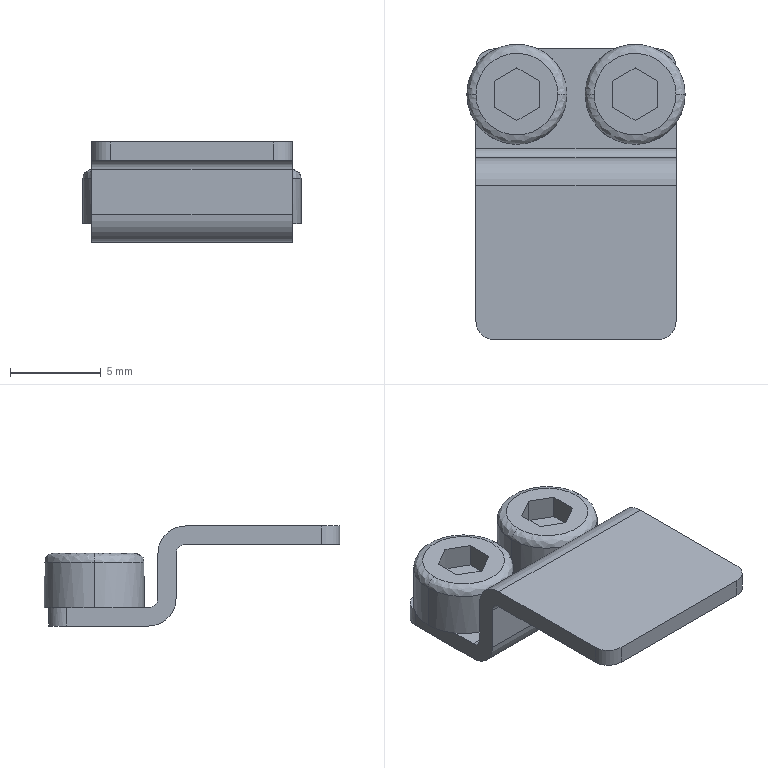Part | SolidWorks | features BaseBody 1 | 1 solid | 54 faces | box 12 x 16.25 x 5.5 mm | volume 322.658 mm3 | plane 34 | cylinder 16 | spline 4 | commonest cylinder face diameters 2 x4 3.5 x4 5.5 x4 1 x2 3 x2